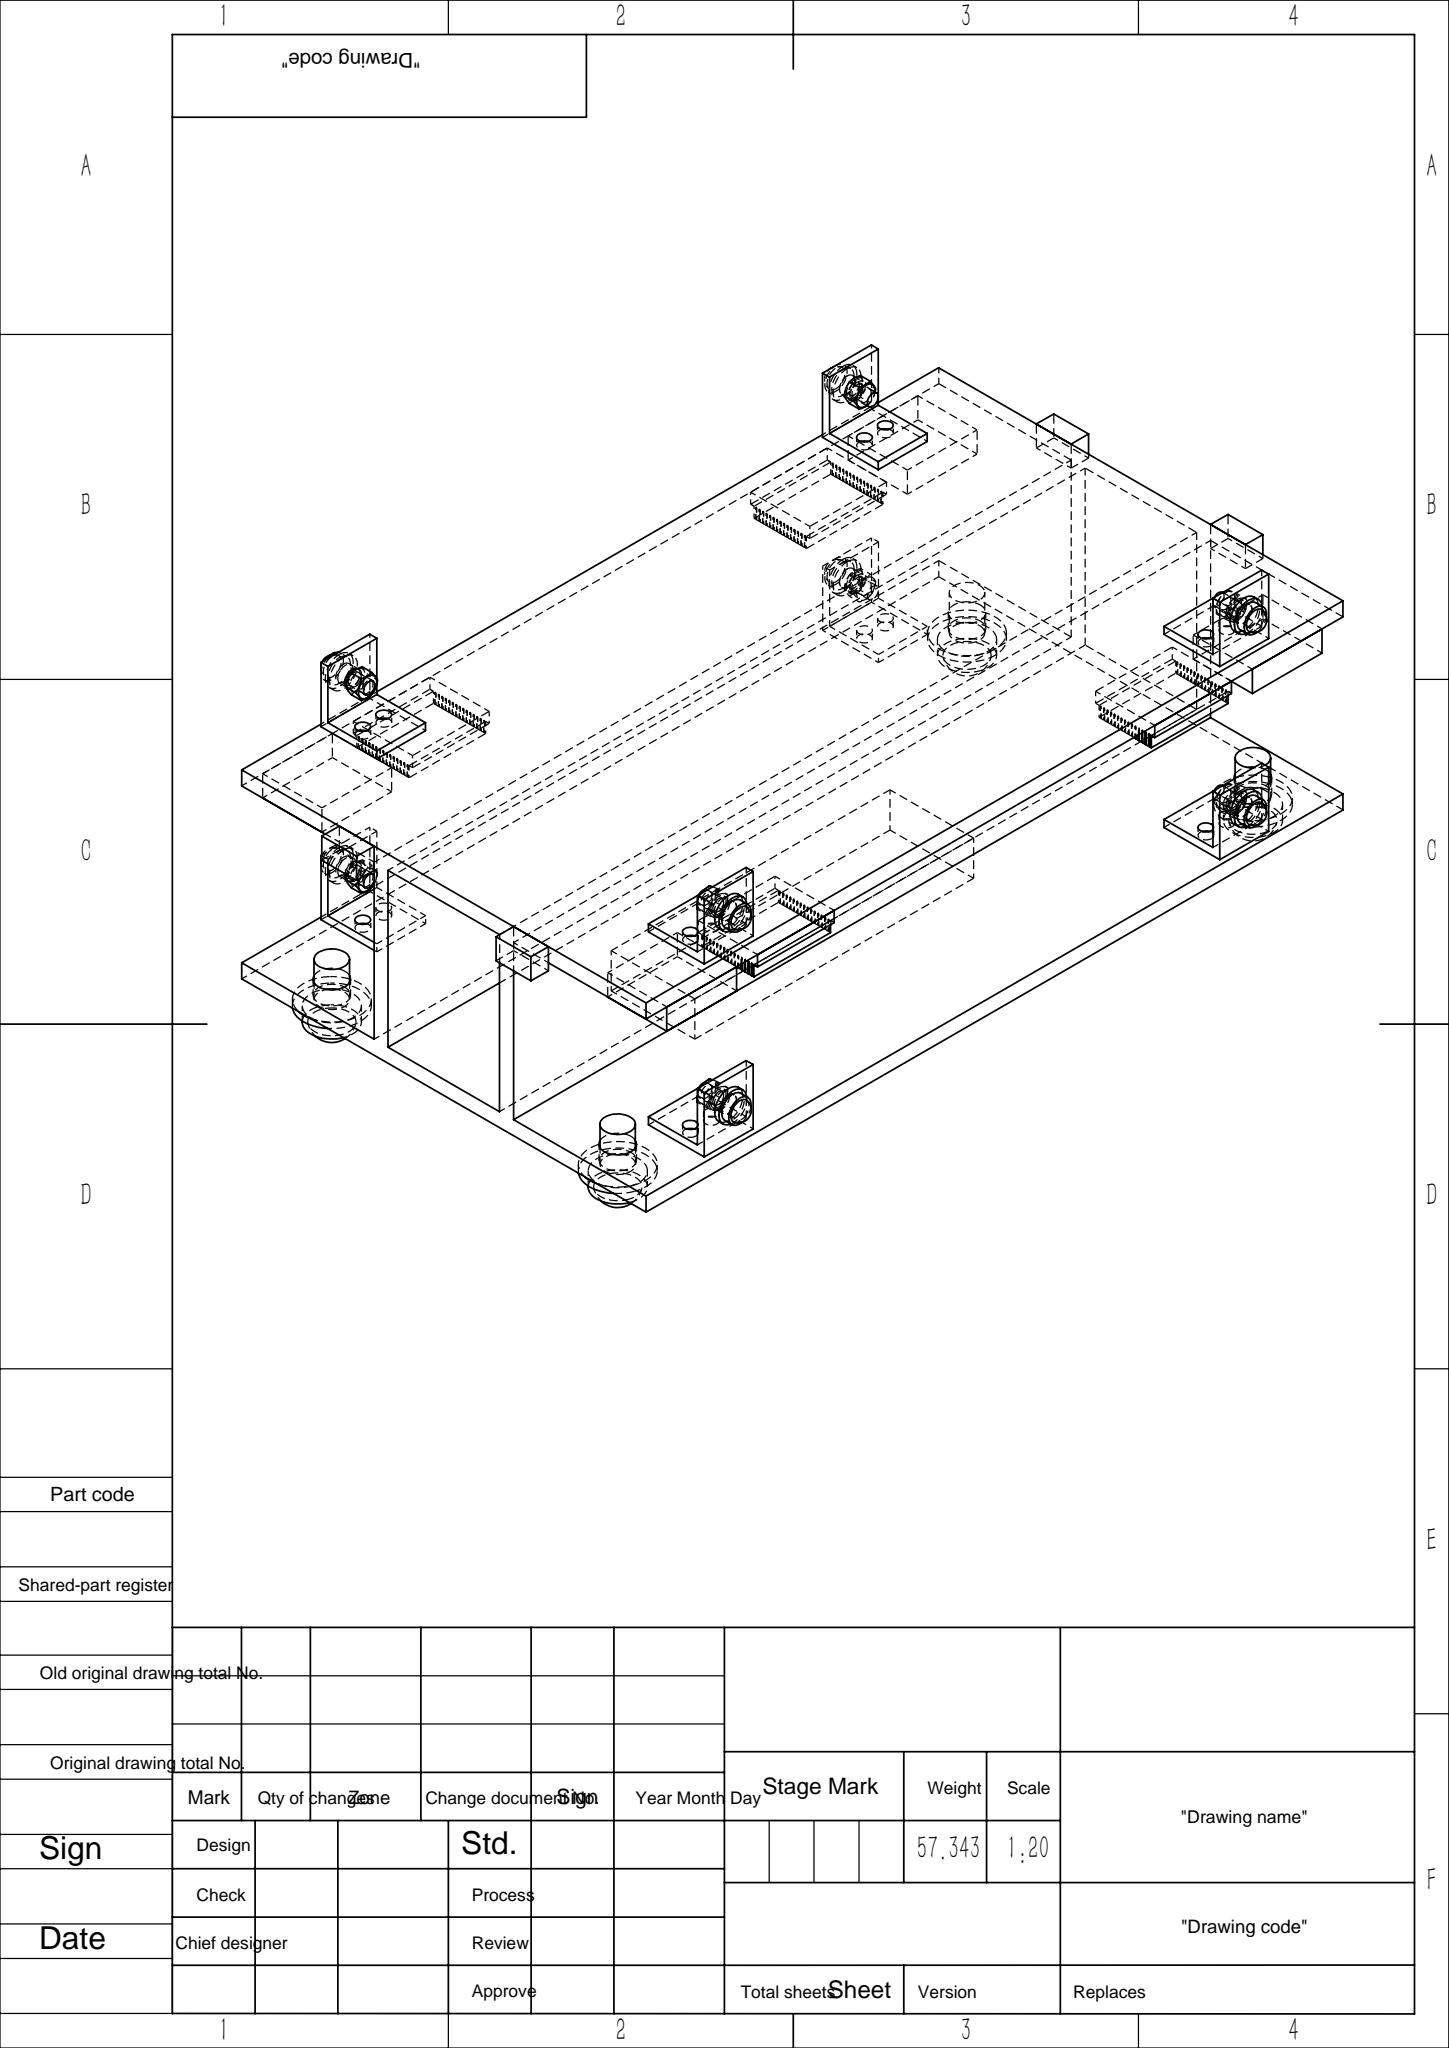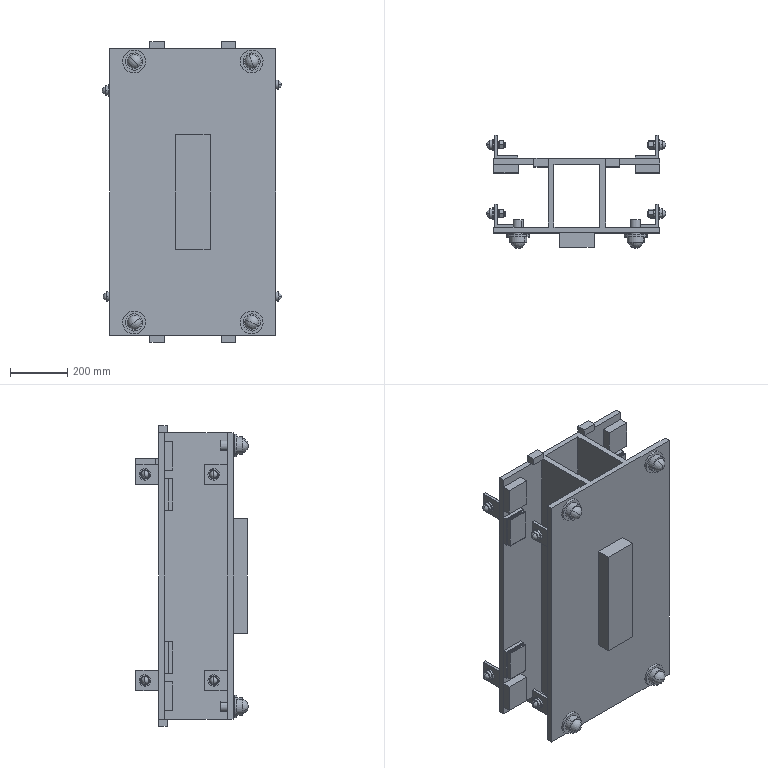Part | SolidWorks | features ReferencePattern 12, LocalLPattern 1 | 42 solids | 1024 faces | box 626.912 x 393.248 x 1050 mm | volume 38288962 mm3 | plane 808 | cylinder 160 | cone 32 | sphere 24 | commonest cylinder face diameters 16 x48 22 x32 15.294 x16 32 x16 40 x16 36 x8